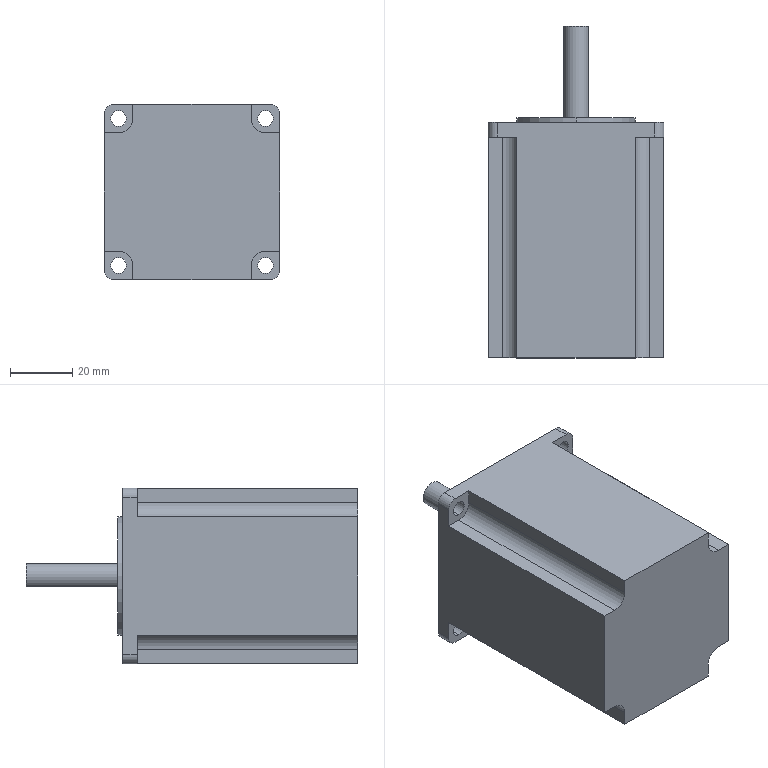Part | SolidWorks | features BaseBody 1 | 1 solid | 40 faces | box 56.4 x 106.5 x 56.4 mm | volume 220040 mm3 | plane 21 | cylinder 19 | commonest cylinder face diameters 5 x8 6 x4 9.26 x4 38.1 x2 8 x1
STEP:
#1=CARTESIAN_POINT('',(1.936,77.1,-3.5));
#2=VERTEX_POINT('',#1);
#3=CARTESIAN_POINT('',(-1.936,77.1,-3.5));
#4=VERTEX_POINT('',#3);
#5=CARTESIAN_POINT('',(1.936,77.1,-3.5));
#6=DIRECTION('',(-1.,0.,0.));
#7=VECTOR('',#6,1000.);
#8=LINE('',#5,#7);
#9=EDGE_CURVE('',#2,#4,#8,.T.);
#10=ORIENTED_EDGE('',*,*,#9,.T.);
#11=CARTESIAN_POINT('',(-1.936,106.5,-3.5));
#12=VERTEX_POINT('',#11);
#13=CARTESIAN_POINT('',(-1.936,73.195,-3.5));
#14=DIRECTION('',(0.,1.,0.));
#15=VECTOR('',#14,1000.);
#16=LINE('',#13,#15);
#17=EDGE_CURVE('',#4,#12,#16,.T.);
#18=ORIENTED_EDGE('',*,*,#17,.T.);
#19=CARTESIAN_POINT('',(1.936,106.5,-3.5));
#20=VERTEX_POINT('',#19);
#21=CARTESIAN_POINT('',(1.936,106.5,-3.5));
#22=DIRECTION('',(1.,0.,0.));
#23=VECTOR('',#22,1000.);
#24=LINE('',#21,#23);
#25=EDGE_CURVE('',#12,#20,#24,.T.);
#26=ORIENTED_EDGE('',*,*,#25,.T.);
#27=CARTESIAN_POINT('',(1.936,73.195,-3.5));
#28=DIRECTION('',(0.,1.,0.));
#29=VECTOR('',#28,1000.);
#30=LINE('',#27,#29);
#31=EDGE_CURVE('',#2,#20,#30,.T.);
#32=ORIENTED_EDGE('',*,*,#31,.F.);
#33=EDGE_LOOP('',(#10,#18,#26,#32));
#34=FACE_OUTER_BOUND('',#33,.T.);
#35=CARTESIAN_POINT('',(1.936,73.195,-3.5));
#36=DIRECTION('',(0.,0.,1.));
#37=DIRECTION('',(1.,0.,0.));
#38=AXIS2_PLACEMENT_3D('',#35,#36,#37);
#39=PLANE('',#38);
#40=ADVANCED_FACE('',(#34),#39,.F.);
#41=CARTESIAN_POINT('',(23.57,70.8,21.07));
#42=VERTEX_POINT('',#41);
#43=CARTESIAN_POINT('',(23.57,75.5,21.07));
#44=VERTEX_POINT('',#43);
#45=CARTESIAN_POINT('',(23.57,0.,21.07));
#46=DIRECTION('',(0.,1.,0.));
#47=VECTOR('',#46,1000.);
#48=LINE('',#45,#47);
#49=EDGE_CURVE('',#42,#44,#48,.T.);
#50=ORIENTED_EDGE('',*,*,#49,.F.);
#51=CARTESIAN_POINT('',(23.57,70.8,26.07));
#52=VERTEX_POINT('',#51);
#53=CARTESIAN_POINT('',(23.57,70.8,23.57));
#54=DIRECTION('',(0.,1.,0.));
#55=DIRECTION('',(0.,0.,1.));
#56=AXIS2_PLACEMENT_3D('',#53,#54,#55);
#57=CIRCLE('',#56,2.5);
#58=EDGE_CURVE('',#52,#42,#57,.T.);
#59=ORIENTED_EDGE('',*,*,#58,.F.);
#60=CARTESIAN_POINT('',(23.57,75.5,26.07));
#61=VERTEX_POINT('',#60);
#62=CARTESIAN_POINT('',(23.57,0.,26.07));
#63=DIRECTION('',(0.,1.,0.));
#64=VECTOR('',#63,1000.);
#65=LINE('',#62,#64);
#66=EDGE_CURVE('',#52,#61,#65,.T.);
#67=ORIENTED_EDGE('',*,*,#66,.T.);
#68=CARTESIAN_POINT('',(23.57,75.5,23.57));
#69=DIRECTION('',(0.,1.,0.));
#70=DIRECTION('',(0.,0.,1.));
#71=AXIS2_PLACEMENT_3D('',#68,#69,#70);
#72=CIRCLE('',#71,2.5);
#73=EDGE_CURVE('',#61,#44,#72,.T.);
#74=ORIENTED_EDGE('',*,*,#73,.T.);
#75=EDGE_LOOP('',(#50,#59,#67,#74));
#76=FACE_OUTER_BOUND('',#75,.T.);
#77=CARTESIAN_POINT('',(23.57,0.,23.57));
#78=DIRECTION('',(0.,1.,0.));
#79=DIRECTION('',(0.,0.,1.));
#80=AXIS2_PLACEMENT_3D('',#77,#78,#79);
#81=CYLINDRICAL_SURFACE('',#80,2.5);
#82=ADVANCED_FACE('',(#76),#81,.F.);
#83=CARTESIAN_POINT('',(-23.57,70.8,-26.07));
#84=VERTEX_POINT('',#83);
#85=CARTESIAN_POINT('',(-23.57,75.5,-26.07));
#86=VERTEX_POINT('',#85);
#87=CARTESIAN_POINT('',(-23.57,0.,-26.07));
#88=DIRECTION('',(0.,1.,0.));
#89=VECTOR('',#88,1000.);
#90=LINE('',#87,#89);
#91=EDGE_CURVE('',#84,#86,#90,.T.);
#92=ORIENTED_EDGE('',*,*,#91,.F.);
#93=CARTESIAN_POINT('',(-23.57,70.8,-21.07));
#94=VERTEX_POINT('',#93);
#95=CARTESIAN_POINT('',(-23.57,70.8,-23.57));
#96=DIRECTION('',(0.,1.,0.));
#97=DIRECTION('',(0.,0.,1.));
#98=AXIS2_PLACEMENT_3D('',#95,#96,#97);
#99=CIRCLE('',#98,2.5);
#100=EDGE_CURVE('',#94,#84,#99,.T.);
#101=ORIENTED_EDGE('',*,*,#100,.F.);
#102=CARTESIAN_POINT('',(-23.57,75.5,-21.07));
#103=VERTEX_POINT('',#102);
#104=CARTESIAN_POINT('',(-23.57,0.,-21.07));
#105=DIRECTION('',(0.,1.,0.));
#106=VECTOR('',#105,1000.);
#107=LINE('',#104,#106);
#108=EDGE_CURVE('',#94,#103,#107,.T.);
#109=ORIENTED_EDGE('',*,*,#108,.T.);
#110=CARTESIAN_POINT('',(-23.57,75.5,-23.57));
#111=DIRECTION('',(0.,1.,0.));
#112=DIRECTION('',(0.,0.,1.));
#113=AXIS2_PLACEMENT_3D('',#110,#111,#112);
#114=CIRCLE('',#113,2.5);
#115=EDGE_CURVE('',#103,#86,#114,.T.);
#116=ORIENTED_EDGE('',*,*,#115,.T.);
#117=EDGE_LOOP('',(#92,#101,#109,#116));
#118=FACE_OUTER_BOUND('',#117,.T.);
#119=CARTESIAN_POINT('',(-23.57,0.,-23.57));
#120=DIRECTION('',(0.,1.,0.));
#121=DIRECTION('',(0.,0.,1.));
#122=AXIS2_PLACEMENT_3D('',#119,#120,#121);
#123=CYLINDRICAL_SURFACE('',#122,2.5);
#124=ADVANCED_FACE('',(#118),#123,.F.);
#125=CARTESIAN_POINT('',(23.57,70.8,-26.07));
#126=VERTEX_POINT('',#125);
#127=CARTESIAN_POINT('',(23.57,75.5,-26.07));
#128=VERTEX_POINT('',#127);
#129=CARTESIAN_POINT('',(23.57,0.,-26.07));
#130=DIRECTION('',(0.,1.,0.));
#131=VECTOR('',#130,1000.);
#132=LINE('',#129,#131);
#133=EDGE_CURVE('',#126,#128,#132,.T.);
#134=ORIENTED_EDGE('',*,*,#133,.F.);
#135=CARTESIAN_POINT('',(23.57,70.8,-21.07));
#136=VERTEX_POINT('',#135);
#137=CARTESIAN_POINT('',(23.57,70.8,-23.57));
#138=DIRECTION('',(0.,-1.,0.));
#139=DIRECTION('',(0.,0.,-1.));
#140=AXIS2_PLACEMENT_3D('',#137,#138,#139);
#141=CIRCLE('',#140,2.5);
#142=EDGE_CURVE('',#126,#136,#141,.T.);
#143=ORIENTED_EDGE('',*,*,#142,.T.);
#144=CARTESIAN_POINT('',(23.57,75.5,-21.07));
#145=VERTEX_POINT('',#144);
#146=CARTESIAN_POINT('',(23.57,0.,-21.07));
#147=DIRECTION('',(0.,1.,0.));
#148=VECTOR('',#147,1000.);
#149=LINE('',#146,#148);
#150=EDGE_CURVE('',#136,#145,#149,.T.);
#151=ORIENTED_EDGE('',*,*,#150,.T.);
#152=CARTESIAN_POINT('',(23.57,75.5,-23.57));
#153=DIRECTION('',(0.,1.,0.));
#154=DIRECTION('',(0.,0.,-1.));
#155=AXIS2_PLACEMENT_3D('',#152,#153,#154);
#156=CIRCLE('',#155,2.5);
#157=EDGE_CURVE('',#145,#128,#156,.T.);
#158=ORIENTED_EDGE('',*,*,#157,.T.);
#159=EDGE_LOOP('',(#134,#143,#151,#158));
#160=FACE_OUTER_BOUND('',#159,.T.);
#161=CARTESIAN_POINT('',(23.57,0.,-23.57));
#162=DIRECTION('',(0.,1.,0.));
#163=DIRECTION('',(0.,0.,1.));
#164=AXIS2_PLACEMENT_3D('',#161,#162,#163);
#165=CYLINDRICAL_SURFACE('',#164,2.5);
#166=ADVANCED_FACE('',(#160),#165,.F.);
#167=CARTESIAN_POINT('',(-23.57,70.8,21.07));
#168=VERTEX_POINT('',#167);
#169=CARTESIAN_POINT('',(-23.57,75.5,21.07));
#170=VERTEX_POINT('',#169);
#171=CARTESIAN_POINT('',(-23.57,0.,21.07));
#172=DIRECTION('',(0.,1.,0.));
#173=VECTOR('',#172,1000.);
#174=LINE('',#171,#173);
#175=EDGE_CURVE('',#168,#170,#174,.T.);
#176=ORIENTED_EDGE('',*,*,#175,.F.);
#177=CARTESIAN_POINT('',(-23.57,70.8,26.07));
#178=VERTEX_POINT('',#177);
#179=CARTESIAN_POINT('',(-23.57,70.8,23.57));
#180=DIRECTION('',(0.,-1.,0.));
#181=DIRECTION('',(0.,0.,-1.));
#182=AXIS2_PLACEMENT_3D('',#179,#180,#181);
#183=CIRCLE('',#182,2.5);
#184=EDGE_CURVE('',#168,#178,#183,.T.);
#185=ORIENTED_EDGE('',*,*,#184,.T.);
#186=CARTESIAN_POINT('',(-23.57,75.5,26.07));
#187=VERTEX_POINT('',#186);
#188=CARTESIAN_POINT('',(-23.57,0.,26.07));
#189=DIRECTION('',(0.,1.,0.));
#190=VECTOR('',#189,1000.);
#191=LINE('',#188,#190);
#192=EDGE_CURVE('',#178,#187,#191,.T.);
#193=ORIENTED_EDGE('',*,*,#192,.T.);
#194=CARTESIAN_POINT('',(-23.57,75.5,23.57));
#195=DIRECTION('',(0.,1.,0.));
#196=DIRECTION('',(0.,0.,-1.));
#197=AXIS2_PLACEMENT_3D('',#194,#195,#196);
#198=CIRCLE('',#197,2.5);
#199=EDGE_CURVE('',#187,#170,#198,.T.);
#200=ORIENTED_EDGE('',*,*,#199,.T.);
#201=EDGE_LOOP('',(#176,#185,#193,#200));
#202=FACE_OUTER_BOUND('',#201,.T.);
#203=CARTESIAN_POINT('',(-23.57,0.,23.57));
#204=DIRECTION('',(0.,1.,0.));
#205=DIRECTION('',(0.,0.,1.));
#206=AXIS2_PLACEMENT_3D('',#203,#204,#205);
#207=CYLINDRICAL_SURFACE('',#206,2.5);
#208=ADVANCED_FACE('',(#202),#207,.F.);
#209=CARTESIAN_POINT('',(-28.2,75.5,25.2));
#210=VERTEX_POINT('',#209);
#211=CARTESIAN_POINT('',(-25.2,75.5,28.2));
#212=VERTEX_POINT('',#211);
#213=CARTESIAN_POINT('',(-25.2,75.5,25.2));
#214=DIRECTION('',(0.,1.,0.));
#215=DIRECTION('',(0.,0.,1.));
#216=AXIS2_PLACEMENT_3D('',#213,#214,#215);
#217=CIRCLE('',#216,3.);
#218=EDGE_CURVE('',#210,#212,#217,.T.);
#219=ORIENTED_EDGE('',*,*,#218,.F.);
#220=CARTESIAN_POINT('',(-28.2,70.8,25.2));
#221=VERTEX_POINT('',#220);
#222=CARTESIAN_POINT('',(-28.2,75.5,25.2));
#223=DIRECTION('',(0.,1.,0.));
#224=VECTOR('',#223,1000.);
#225=LINE('',#222,#224);
#226=EDGE_CURVE('',#221,#210,#225,.T.);
#227=ORIENTED_EDGE('',*,*,#226,.F.);
#228=CARTESIAN_POINT('',(-25.2,70.8,28.2));
#229=VERTEX_POINT('',#228);
#230=CARTESIAN_POINT('',(-25.2,70.8,25.2));
#231=DIRECTION('',(0.,-1.,0.));
#232=DIRECTION('',(0.,0.,-1.));
#233=AXIS2_PLACEMENT_3D('',#230,#231,#232);
#234=CIRCLE('',#233,3.);
#235=EDGE_CURVE('',#229,#221,#234,.T.);
#236=ORIENTED_EDGE('',*,*,#235,.F.);
#237=CARTESIAN_POINT('',(-25.2,75.5,28.2));
#238=DIRECTION('',(0.,-1.,0.));
#239=VECTOR('',#238,1000.);
#240=LINE('',#237,#239);
#241=EDGE_CURVE('',#212,#229,#240,.T.);
#242=ORIENTED_EDGE('',*,*,#241,.F.);
#243=EDGE_LOOP('',(#219,#227,#236,#242));
#244=FACE_OUTER_BOUND('',#243,.T.);
#245=CARTESIAN_POINT('',(-25.2,75.5,25.2));
#246=DIRECTION('',(0.,-1.,0.));
#247=DIRECTION('',(0.,0.,-1.));
#248=AXIS2_PLACEMENT_3D('',#245,#246,#247);
#249=CYLINDRICAL_SURFACE('',#248,3.);
#250=ADVANCED_FACE('',(#244),#249,.T.);
#251=CARTESIAN_POINT('',(-25.2,75.5,-28.2));
#252=VERTEX_POINT('',#251);
#253=CARTESIAN_POINT('',(-28.2,75.5,-25.2));
#254=VERTEX_POINT('',#253);
#255=CARTESIAN_POINT('',(-25.2,75.5,-25.2));
#256=DIRECTION('',(0.,1.,0.));
#257=DIRECTION('',(0.,0.,1.));
#258=AXIS2_PLACEMENT_3D('',#255,#256,#257);
#259=CIRCLE('',#258,3.);
#260=EDGE_CURVE('',#252,#254,#259,.T.);
#261=ORIENTED_EDGE('',*,*,#260,.F.);
#262=CARTESIAN_POINT('',(-25.2,70.8,-28.2));
#263=VERTEX_POINT('',#262);
#264=CARTESIAN_POINT('',(-25.2,75.5,-28.2));
#265=DIRECTION('',(0.,1.,0.));
#266=VECTOR('',#265,1000.);
#267=LINE('',#264,#266);
#268=EDGE_CURVE('',#263,#252,#267,.T.);
#269=ORIENTED_EDGE('',*,*,#268,.F.);
#270=CARTESIAN_POINT('',(-28.2,70.8,-25.2));
#271=VERTEX_POINT('',#270);
#272=CARTESIAN_POINT('',(-25.2,70.8,-25.2));
#273=DIRECTION('',(0.,-1.,0.));
#274=DIRECTION('',(0.,0.,1.));
#275=AXIS2_PLACEMENT_3D('',#272,#273,#274);
#276=CIRCLE('',#275,3.);
#277=EDGE_CURVE('',#271,#263,#276,.T.);
#278=ORIENTED_EDGE('',*,*,#277,.F.);
#279=CARTESIAN_POINT('',(-28.2,75.5,-25.2));
#280=DIRECTION('',(0.,-1.,0.));
#281=VECTOR('',#280,1000.);
#282=LINE('',#279,#281);
#283=EDGE_CURVE('',#254,#271,#282,.T.);
#284=ORIENTED_EDGE('',*,*,#283,.F.);
#285=EDGE_LOOP('',(#261,#269,#278,#284));
#286=FACE_OUTER_BOUND('',#285,.T.);
#287=CARTESIAN_POINT('',(-25.2,75.5,-25.2));
#288=DIRECTION('',(0.,-1.,0.));
#289=DIRECTION('',(0.,0.,-1.));
#290=AXIS2_PLACEMENT_3D('',#287,#288,#289);
#291=CYLINDRICAL_SURFACE('',#290,3.);
#292=ADVANCED_FACE('',(#286),#291,.T.);
#293=CARTESIAN_POINT('',(25.2,75.5,28.2));
#294=VERTEX_POINT('',#293);
#295=CARTESIAN_POINT('',(28.2,75.5,25.2));
#296=VERTEX_POINT('',#295);
#297=CARTESIAN_POINT('',(25.2,75.5,25.2));
#298=DIRECTION('',(0.,1.,0.));
#299=DIRECTION('',(0.,0.,1.));
#300=AXIS2_PLACEMENT_3D('',#297,#298,#299);
#301=CIRCLE('',#300,3.);
#302=EDGE_CURVE('',#294,#296,#301,.T.);
#303=ORIENTED_EDGE('',*,*,#302,.F.);
#304=CARTESIAN_POINT('',(25.2,70.8,28.2));
#305=VERTEX_POINT('',#304);
#306=CARTESIAN_POINT('',(25.2,75.5,28.2));
#307=DIRECTION('',(0.,1.,0.));
#308=VECTOR('',#307,1000.);
#309=LINE('',#306,#308);
#310=EDGE_CURVE('',#305,#294,#309,.T.);
#311=ORIENTED_EDGE('',*,*,#310,.F.);
#312=CARTESIAN_POINT('',(28.2,70.8,25.2));
#313=VERTEX_POINT('',#312);
#314=CARTESIAN_POINT('',(25.2,70.8,25.2));
#315=DIRECTION('',(0.,-1.,0.));
#316=DIRECTION('',(0.,0.,1.));
#317=AXIS2_PLACEMENT_3D('',#314,#315,#316);
#318=CIRCLE('',#317,3.);
#319=EDGE_CURVE('',#313,#305,#318,.T.);
#320=ORIENTED_EDGE('',*,*,#319,.F.);
#321=CARTESIAN_POINT('',(28.2,75.5,25.2));
#322=DIRECTION('',(0.,-1.,0.));
#323=VECTOR('',#322,1000.);
#324=LINE('',#321,#323);
#325=EDGE_CURVE('',#296,#313,#324,.T.);
#326=ORIENTED_EDGE('',*,*,#325,.F.);
#327=EDGE_LOOP('',(#303,#311,#320,#326));
#328=FACE_OUTER_BOUND('',#327,.T.);
#329=CARTESIAN_POINT('',(25.2,75.5,25.2));
#330=DIRECTION('',(0.,-1.,0.));
#331=DIRECTION('',(0.,0.,-1.));
#332=AXIS2_PLACEMENT_3D('',#329,#330,#331);
#333=CYLINDRICAL_SURFACE('',#332,3.);
#334=ADVANCED_FACE('',(#328),#333,.T.);
#335=CARTESIAN_POINT('',(28.2,75.5,-25.2));
#336=VERTEX_POINT('',#335);
#337=CARTESIAN_POINT('',(25.2,75.5,-28.2));
#338=VERTEX_POINT('',#337);
#339=CARTESIAN_POINT('',(25.2,75.5,-25.2));
#340=DIRECTION('',(0.,1.,0.));
#341=DIRECTION('',(0.,0.,1.));
#342=AXIS2_PLACEMENT_3D('',#339,#340,#341);
#343=CIRCLE('',#342,3.);
#344=EDGE_CURVE('',#336,#338,#343,.T.);
#345=ORIENTED_EDGE('',*,*,#344,.F.);
#346=CARTESIAN_POINT('',(28.2,70.8,-25.2));
#347=VERTEX_POINT('',#346);
#348=CARTESIAN_POINT('',(28.2,75.5,-25.2));
#349=DIRECTION('',(0.,1.,0.));
#350=VECTOR('',#349,1000.);
#351=LINE('',#348,#350);
#352=EDGE_CURVE('',#347,#336,#351,.T.);
#353=ORIENTED_EDGE('',*,*,#352,.F.);
#354=CARTESIAN_POINT('',(25.2,70.8,-28.2));
#355=VERTEX_POINT('',#354);
#356=CARTESIAN_POINT('',(25.2,70.8,-25.2));
#357=DIRECTION('',(0.,-1.,0.));
#358=DIRECTION('',(0.,0.,-1.));
#359=AXIS2_PLACEMENT_3D('',#356,#357,#358);
#360=CIRCLE('',#359,3.);
#361=EDGE_CURVE('',#355,#347,#360,.T.);
#362=ORIENTED_EDGE('',*,*,#361,.F.);
#363=CARTESIAN_POINT('',(25.2,75.5,-28.2));
#364=DIRECTION('',(0.,-1.,0.));
#365=VECTOR('',#364,1000.);
#366=LINE('',#363,#365);
#367=EDGE_CURVE('',#338,#355,#366,.T.);
#368=ORIENTED_EDGE('',*,*,#367,.F.);
#369=EDGE_LOOP('',(#345,#353,#362,#368));
#370=FACE_OUTER_BOUND('',#369,.T.);
#371=CARTESIAN_POINT('',(25.2,75.5,-25.2));
#372=DIRECTION('',(0.,-1.,0.));
#373=DIRECTION('',(0.,0.,-1.));
#374=AXIS2_PLACEMENT_3D('',#371,#372,#373);
#375=CYLINDRICAL_SURFACE('',#374,3.);
#376=ADVANCED_FACE('',(#370),#375,.T.);
#377=CARTESIAN_POINT('',(-23.57,70.8,23.57));
#378=DIRECTION('',(0.,-1.,0.));
#379=DIRECTION('',(0.,0.,-1.));
#380=AXIS2_PLACEMENT_3D('',#377,#378,#379);
#381=CIRCLE('',#380,2.5);
#382=EDGE_CURVE('',#178,#168,#381,.T.);
#383=ORIENTED_EDGE('',*,*,#382,.F.);
#384=ORIENTED_EDGE('',*,*,#184,.F.);
#385=EDGE_LOOP('',(#383,#384));
#386=FACE_BOUND('',#385,.T.);
#387=CARTESIAN_POINT('',(-18.94,70.8,28.2));
#388=VERTEX_POINT('',#387);
#389=CARTESIAN_POINT('',(-28.2,70.8,28.2));
#390=DIRECTION('',(-1.,0.,0.));
#391=VECTOR('',#390,1000.);
#392=LINE('',#389,#391);
#393=EDGE_CURVE('',#388,#229,#392,.T.);
#394=ORIENTED_EDGE('',*,*,#393,.T.);
#395=ORIENTED_EDGE('',*,*,#235,.T.);
#396=CARTESIAN_POINT('',(-28.2,70.8,18.94));
#397=VERTEX_POINT('',#396);
#398=CARTESIAN_POINT('',(-28.2,70.8,18.94));
#399=DIRECTION('',(0.,0.,-1.));
#400=VECTOR('',#399,1000.);
#401=LINE('',#398,#400);
#402=EDGE_CURVE('',#221,#397,#401,.T.);
#403=ORIENTED_EDGE('',*,*,#402,.T.);
#404=CARTESIAN_POINT('',(-23.57,70.8,18.94));
#405=VERTEX_POINT('',#404);
#406=CARTESIAN_POINT('',(-23.57,70.8,18.94));
#407=DIRECTION('',(1.,0.,0.));
#408=VECTOR('',#407,1000.);
#409=LINE('',#406,#408);
#410=EDGE_CURVE('',#397,#405,#409,.T.);
#411=ORIENTED_EDGE('',*,*,#410,.T.);
#412=CARTESIAN_POINT('',(-18.94,70.8,23.57));
#413=VERTEX_POINT('',#412);
#414=CARTESIAN_POINT('',(-23.57,70.8,23.57));
#415=DIRECTION('',(0.,-1.,0.));
#416=DIRECTION('',(0.,0.,-1.));
#417=AXIS2_PLACEMENT_3D('',#414,#415,#416);
#418=CIRCLE('',#417,4.63);
#419=EDGE_CURVE('',#405,#413,#418,.T.);
#420=ORIENTED_EDGE('',*,*,#419,.T.);
#421=CARTESIAN_POINT('',(-18.94,70.8,23.57));
#422=DIRECTION('',(0.,0.,1.));
#423=VECTOR('',#422,1000.);
#424=LINE('',#421,#423);
#425=EDGE_CURVE('',#413,#388,#424,.T.);
#426=ORIENTED_EDGE('',*,*,#425,.T.);
#427=EDGE_LOOP('',(#394,#395,#403,#411,#420,#426));
#428=FACE_OUTER_BOUND('',#427,.T.);
#429=CARTESIAN_POINT('',(-23.57,70.8,23.57));
#430=DIRECTION('',(0.,-1.,0.));
#431=DIRECTION('',(0.,0.,-1.));
#432=AXIS2_PLACEMENT_3D('',#429,#430,#431);
#433=PLANE('',#432);
#434=ADVANCED_FACE('',(#386,#428),#433,.T.);
#435=CARTESIAN_POINT('',(-18.94,0.,23.57));
#436=VERTEX_POINT('',#435);
#437=CARTESIAN_POINT('',(-18.94,0.,28.2));
#438=VERTEX_POINT('',#437);
#439=CARTESIAN_POINT('',(-18.94,0.,23.57));
#440=DIRECTION('',(0.,0.,1.));
#441=VECTOR('',#440,1000.);
#442=LINE('',#439,#441);
#443=EDGE_CURVE('',#436,#438,#442,.T.);
#444=ORIENTED_EDGE('',*,*,#443,.T.);
#445=CARTESIAN_POINT('',(-18.94,70.8,28.2));
#446=DIRECTION('',(0.,-1.,0.));
#447=VECTOR('',#446,1000.);
#448=LINE('',#445,#447);
#449=EDGE_CURVE('',#388,#438,#448,.T.);
#450=ORIENTED_EDGE('',*,*,#449,.F.);
#451=ORIENTED_EDGE('',*,*,#425,.F.);
#452=CARTESIAN_POINT('',(-18.94,70.8,23.57));
#453=DIRECTION('',(0.,-1.,0.));
#454=VECTOR('',#453,1000.);
#455=LINE('',#452,#454);
#456=EDGE_CURVE('',#413,#436,#455,.T.);
#457=ORIENTED_EDGE('',*,*,#456,.T.);
#458=EDGE_LOOP('',(#444,#450,#451,#457));
#459=FACE_OUTER_BOUND('',#458,.T.);
#460=CARTESIAN_POINT('',(-18.94,70.8,23.57));
#461=DIRECTION('',(1.,0.,0.));
#462=DIRECTION('',(0.,0.,1.));
#463=AXIS2_PLACEMENT_3D('',#460,#461,#462);
#464=PLANE('',#463);
#465=ADVANCED_FACE('',(#459),#464,.F.);
#466=CARTESIAN_POINT('',(-28.2,0.,18.94));
#467=VERTEX_POINT('',#466);
#468=CARTESIAN_POINT('',(-23.57,0.,18.94));
#469=VERTEX_POINT('',#468);
#470=CARTESIAN_POINT('',(-23.57,0.,18.94));
#471=DIRECTION('',(1.,0.,0.));
#472=VECTOR('',#471,1000.);
#473=LINE('',#470,#472);
#474=EDGE_CURVE('',#467,#469,#473,.T.);
#475=ORIENTED_EDGE('',*,*,#474,.T.);
#476=CARTESIAN_POINT('',(-23.57,70.8,18.94));
#477=DIRECTION('',(0.,-1.,0.));
#478=VECTOR('',#477,1000.);
#479=LINE('',#476,#478);
#480=EDGE_CURVE('',#405,#469,#479,.T.);
#481=ORIENTED_EDGE('',*,*,#480,.F.);
#482=ORIENTED_EDGE('',*,*,#410,.F.);
#483=CARTESIAN_POINT('',(-28.2,70.8,18.94));
#484=DIRECTION('',(0.,-1.,0.));
#485=VECTOR('',#484,1000.);
#486=LINE('',#483,#485);
#487=EDGE_CURVE('',#397,#467,#486,.T.);
#488=ORIENTED_EDGE('',*,*,#487,.T.);
#489=EDGE_LOOP('',(#475,#481,#482,#488));
#490=FACE_OUTER_BOUND('',#489,.T.);
#491=CARTESIAN_POINT('',(-23.57,70.8,18.94));
#492=DIRECTION('',(0.,0.,-1.));
#493=DIRECTION('',(0.,-1.,0.));
#494=AXIS2_PLACEMENT_3D('',#491,#492,#493);
#495=PLANE('',#494);
#496=ADVANCED_FACE('',(#490),#495,.F.);
#497=CARTESIAN_POINT('',(-23.57,0.,23.57));
#498=DIRECTION('',(0.,-1.,0.));
#499=DIRECTION('',(0.,0.,-1.));
#500=AXIS2_PLACEMENT_3D('',#497,#498,#499);
#501=CIRCLE('',#500,4.63);
#502=EDGE_CURVE('',#469,#436,#501,.T.);
#503=ORIENTED_EDGE('',*,*,#502,.T.);
#504=ORIENTED_EDGE('',*,*,#456,.F.);
#505=ORIENTED_EDGE('',*,*,#419,.F.);
#506=ORIENTED_EDGE('',*,*,#480,.T.);
#507=EDGE_LOOP('',(#503,#504,#505,#506));
#508=FACE_OUTER_BOUND('',#507,.T.);
#509=CARTESIAN_POINT('',(-23.57,70.8,23.57));
#510=DIRECTION('',(0.,-1.,0.));
#511=DIRECTION('',(0.,0.,-1.));
#512=AXIS2_PLACEMENT_3D('',#509,#510,#511);
#513=CYLINDRICAL_SURFACE('',#512,4.63);
#514=ADVANCED_FACE('',(#508),#513,.F.);
#515=CARTESIAN_POINT('',(23.57,70.8,-23.57));
#516=DIRECTION('',(0.,-1.,0.));
#517=DIRECTION('',(0.,0.,-1.));
#518=AXIS2_PLACEMENT_3D('',#515,#516,#517);
#519=CIRCLE('',#518,2.5);
#520=EDGE_CURVE('',#136,#126,#519,.T.);
#521=ORIENTED_EDGE('',*,*,#520,.F.);
#522=ORIENTED_EDGE('',*,*,#142,.F.);
#523=EDGE_LOOP('',(#521,#522));
#524=FACE_BOUND('',#523,.T.);
#525=CARTESIAN_POINT('',(18.94,70.8,-28.2));
#526=VERTEX_POINT('',#525);
#527=CARTESIAN_POINT('',(28.2,70.8,-28.2));
#528=DIRECTION('',(1.,0.,0.));
#529=VECTOR('',#528,1000.);
#530=LINE('',#527,#529);
#531=EDGE_CURVE('',#526,#355,#530,.T.);
#532=ORIENTED_EDGE('',*,*,#531,.T.);
#533=ORIENTED_EDGE('',*,*,#361,.T.);
#534=CARTESIAN_POINT('',(28.2,70.8,-18.94));
#535=VERTEX_POINT('',#534);
#536=CARTESIAN_POINT('',(28.2,70.8,-18.94));
#537=DIRECTION('',(0.,0.,1.));
#538=VECTOR('',#537,1000.);
#539=LINE('',#536,#538);
#540=EDGE_CURVE('',#347,#535,#539,.T.);
#541=ORIENTED_EDGE('',*,*,#540,.T.);
#542=CARTESIAN_POINT('',(23.57,70.8,-18.94));
#543=VERTEX_POINT('',#542);
#544=CARTESIAN_POINT('',(23.57,70.8,-18.94));
#545=DIRECTION('',(-1.,0.,0.));
#546=VECTOR('',#545,1000.);
#547=LINE('',#544,#546);
#548=EDGE_CURVE('',#535,#543,#547,.T.);
#549=ORIENTED_EDGE('',*,*,#548,.T.);
#550=CARTESIAN_POINT('',(18.94,70.8,-23.57));
#551=VERTEX_POINT('',#550);
#552=CARTESIAN_POINT('',(23.57,70.8,-23.57));
#553=DIRECTION('',(0.,-1.,0.));
#554=DIRECTION('',(0.,0.,-1.));
#555=AXIS2_PLACEMENT_3D('',#552,#553,#554);
#556=CIRCLE('',#555,4.63);
#557=EDGE_CURVE('',#543,#551,#556,.T.);
#558=ORIENTED_EDGE('',*,*,#557,.T.);
#559=CARTESIAN_POINT('',(18.94,70.8,-23.57));
#560=DIRECTION('',(0.,0.,-1.));
#561=VECTOR('',#560,1000.);
#562=LINE('',#559,#561);
#563=EDGE_CURVE('',#551,#526,#562,.T.);
#564=ORIENTED_EDGE('',*,*,#563,.T.);
#565=EDGE_LOOP('',(#532,#533,#541,#549,#558,#564));
#566=FACE_OUTER_BOUND('',#565,.T.);
#567=CARTESIAN_POINT('',(23.57,70.8,-23.57));
#568=DIRECTION('',(0.,-1.,0.));
#569=DIRECTION('',(0.,0.,-1.));
#570=AXIS2_PLACEMENT_3D('',#567,#568,#569);
#571=PLANE('',#570);
#572=ADVANCED_FACE('',(#524,#566),#571,.T.);
#573=CARTESIAN_POINT('',(18.94,0.,-23.57));
#574=VERTEX_POINT('',#573);
#575=CARTESIAN_POINT('',(18.94,0.,-28.2));
#576=VERTEX_POINT('',#575);
#577=CARTESIAN_POINT('',(18.94,0.,-23.57));
#578=DIRECTION('',(0.,0.,-1.));
#579=VECTOR('',#578,1000.);
#580=LINE('',#577,#579);
#581=EDGE_CURVE('',#574,#576,#580,.T.);
#582=ORIENTED_EDGE('',*,*,#581,.T.);
#583=CARTESIAN_POINT('',(18.94,70.8,-28.2));
#584=DIRECTION('',(0.,-1.,0.));
#585=VECTOR('',#584,1000.);
#586=LINE('',#583,#585);
#587=EDGE_CURVE('',#526,#576,#586,.T.);
#588=ORIENTED_EDGE('',*,*,#587,.F.);
#589=ORIENTED_EDGE('',*,*,#563,.F.);
#590=CARTESIAN_POINT('',(18.94,70.8,-23.57));
#591=DIRECTION('',(0.,-1.,0.));
#592=VECTOR('',#591,1000.);
#593=LINE('',#590,#592);
#594=EDGE_CURVE('',#551,#574,#593,.T.);
#595=ORIENTED_EDGE('',*,*,#594,.T.);
#596=EDGE_LOOP('',(#582,#588,#589,#595));
#597=FACE_OUTER_BOUND('',#596,.T.);
#598=CARTESIAN_POINT('',(18.94,70.8,-23.57));
#599=DIRECTION('',(-1.,0.,0.));
#600=DIRECTION('',(0.,0.,1.));
#601=AXIS2_PLACEMENT_3D('',#598,#599,#600);
#602=PLANE('',#601);
#603=ADVANCED_FACE('',(#597),#602,.F.);
#604=CARTESIAN_POINT('',(28.2,0.,-18.94));
#605=VERTEX_POINT('',#604);
#606=CARTESIAN_POINT('',(23.57,0.,-18.94));
#607=VERTEX_POINT('',#606);
#608=CARTESIAN_POINT('',(23.57,0.,-18.94));
#609=DIRECTION('',(-1.,0.,0.));
#610=VECTOR('',#609,1000.);
#611=LINE('',#608,#610);
#612=EDGE_CURVE('',#605,#607,#611,.T.);
#613=ORIENTED_EDGE('',*,*,#612,.T.);
#614=CARTESIAN_POINT('',(23.57,70.8,-18.94));
#615=DIRECTION('',(0.,-1.,0.));
#616=VECTOR('',#615,1000.);
#617=LINE('',#614,#616);
#618=EDGE_CURVE('',#543,#607,#617,.T.);
#619=ORIENTED_EDGE('',*,*,#618,.F.);
#620=ORIENTED_EDGE('',*,*,#548,.F.);
#621=CARTESIAN_POINT('',(28.2,70.8,-18.94));
#622=DIRECTION('',(0.,-1.,0.));
#623=VECTOR('',#622,1000.);
#624=LINE('',#621,#623);
#625=EDGE_CURVE('',#535,#605,#624,.T.);
#626=ORIENTED_EDGE('',*,*,#625,.T.);
#627=EDGE_LOOP('',(#613,#619,#620,#626));
#628=FACE_OUTER_BOUND('',#627,.T.);
#629=CARTESIAN_POINT('',(23.57,70.8,-18.94));
#630=DIRECTION('',(0.,0.,1.));
#631=DIRECTION('',(1.,0.,0.));
#632=AXIS2_PLACEMENT_3D('',#629,#630,#631);
#633=PLANE('',#632);
#634=ADVANCED_FACE('',(#628),#633,.F.);
#635=CARTESIAN_POINT('',(23.57,0.,-23.57));
#636=DIRECTION('',(0.,-1.,0.));
#637=DIRECTION('',(0.,0.,-1.));
#638=AXIS2_PLACEMENT_3D('',#635,#636,#637);
#639=CIRCLE('',#638,4.63);
#640=EDGE_CURVE('',#607,#574,#639,.T.);
#641=ORIENTED_EDGE('',*,*,#640,.T.);
#642=ORIENTED_EDGE('',*,*,#594,.F.);
#643=ORIENTED_EDGE('',*,*,#557,.F.);
#644=ORIENTED_EDGE('',*,*,#618,.T.);
#645=EDGE_LOOP('',(#641,#642,#643,#644));
#646=FACE_OUTER_BOUND('',#645,.T.);
#647=CARTESIAN_POINT('',(23.57,70.8,-23.57));
#648=DIRECTION('',(0.,-1.,0.));
#649=DIRECTION('',(0.,0.,-1.));
#650=AXIS2_PLACEMENT_3D('',#647,#648,#649);
#651=CYLINDRICAL_SURFACE('',#650,4.63);
#652=ADVANCED_FACE('',(#646),#651,.F.);
#653=ORIENTED_EDGE('',*,*,#100,.T.);
#654=CARTESIAN_POINT('',(-23.57,70.8,-23.57));
#655=DIRECTION('',(0.,1.,0.));
#656=DIRECTION('',(0.,0.,1.));
#657=AXIS2_PLACEMENT_3D('',#654,#655,#656);
#658=CIRCLE('',#657,2.5);
#659=EDGE_CURVE('',#84,#94,#658,.T.);
#660=ORIENTED_EDGE('',*,*,#659,.T.);
#661=EDGE_LOOP('',(#653,#660));
#662=FACE_BOUND('',#661,.T.);
#663=CARTESIAN_POINT('',(-28.2,70.8,-18.94));
#664=VERTEX_POINT('',#663);
#665=CARTESIAN_POINT('',(-28.2,70.8,-18.94));
#666=DIRECTION('',(0.,0.,-1.));
#667=VECTOR('',#666,1000.);
#668=LINE('',#665,#667);
#669=EDGE_CURVE('',#664,#271,#668,.T.);
#670=ORIENTED_EDGE('',*,*,#669,.T.);
#671=ORIENTED_EDGE('',*,*,#277,.T.);
#672=CARTESIAN_POINT('',(-18.94,70.8,-28.2));
#673=VERTEX_POINT('',#672);
#674=CARTESIAN_POINT('',(-28.2,70.8,-28.2));
#675=DIRECTION('',(1.,0.,0.));
#676=VECTOR('',#675,1000.);
#677=LINE('',#674,#676);
#678=EDGE_CURVE('',#263,#673,#677,.T.);
#679=ORIENTED_EDGE('',*,*,#678,.T.);
#680=CARTESIAN_POINT('',(-18.94,70.8,-23.57));
#681=VERTEX_POINT('',#680);
#682=CARTESIAN_POINT('',(-18.94,70.8,-23.57));
#683=DIRECTION('',(0.,0.,1.));
#684=VECTOR('',#683,1000.);
#685=LINE('',#682,#684);
#686=EDGE_CURVE('',#673,#681,#685,.T.);
#687=ORIENTED_EDGE('',*,*,#686,.T.);
#688=CARTESIAN_POINT('',(-23.57,70.8,-18.94));
#689=VERTEX_POINT('',#688);
#690=CARTESIAN_POINT('',(-23.57,70.8,-23.57));
#691=DIRECTION('',(0.,-1.,0.));
#692=DIRECTION('',(0.,0.,1.));
#693=AXIS2_PLACEMENT_3D('',#690,#691,#692);
#694=CIRCLE('',#693,4.63);
#695=EDGE_CURVE('',#681,#689,#694,.T.);
#696=ORIENTED_EDGE('',*,*,#695,.T.);
#697=CARTESIAN_POINT('',(-23.57,70.8,-18.94));
#698=DIRECTION('',(-1.,0.,0.));
#699=VECTOR('',#698,1000.);
#700=LINE('',#697,#699);
#701=EDGE_CURVE('',#689,#664,#700,.T.);
#702=ORIENTED_EDGE('',*,*,#701,.T.);
#703=EDGE_LOOP('',(#670,#671,#679,#687,#696,#702));
#704=FACE_OUTER_BOUND('',#703,.T.);
#705=CARTESIAN_POINT('',(-23.57,70.8,-23.57));
#706=DIRECTION('',(0.,1.,0.));
#707=DIRECTION('',(1.,0.,0.));
#708=AXIS2_PLACEMENT_3D('',#705,#706,#707);
#709=PLANE('',#708);
#710=ADVANCED_FACE('',(#662,#704),#709,.F.);
#711=CARTESIAN_POINT('',(-23.57,0.,-18.94));
#712=VERTEX_POINT('',#711);
#713=CARTESIAN_POINT('',(-28.2,0.,-18.94));
#714=VERTEX_POINT('',#713);
#715=CARTESIAN_POINT('',(-23.57,0.,-18.94));
#716=DIRECTION('',(-1.,0.,0.));
#717=VECTOR('',#716,1000.);
#718=LINE('',#715,#717);
#719=EDGE_CURVE('',#712,#714,#718,.T.);
#720=ORIENTED_EDGE('',*,*,#719,.T.);
#721=CARTESIAN_POINT('',(-28.2,70.8,-18.94));
#722=DIRECTION('',(0.,-1.,0.));
#723=VECTOR('',#722,1000.);
#724=LINE('',#721,#723);
#725=EDGE_CURVE('',#664,#714,#724,.T.);
#726=ORIENTED_EDGE('',*,*,#725,.F.);
#727=ORIENTED_EDGE('',*,*,#701,.F.);
#728=CARTESIAN_POINT('',(-23.57,70.8,-18.94));
#729=DIRECTION('',(0.,-1.,0.));
#730=VECTOR('',#729,1000.);
#731=LINE('',#728,#730);
#732=EDGE_CURVE('',#689,#712,#731,.T.);
#733=ORIENTED_EDGE('',*,*,#732,.T.);
#734=EDGE_LOOP('',(#720,#726,#727,#733));
#735=FACE_OUTER_BOUND('',#734,.T.);
#736=CARTESIAN_POINT('',(-23.57,70.8,-18.94));
#737=DIRECTION('',(0.,0.,1.));
#738=DIRECTION('',(1.,0.,0.));
#739=AXIS2_PLACEMENT_3D('',#736,#737,#738);
#740=PLANE('',#739);
#741=ADVANCED_FACE('',(#735),#740,.F.);
#742=CARTESIAN_POINT('',(-18.94,0.,-28.2));
#743=VERTEX_POINT('',#742);
#744=CARTESIAN_POINT('',(-18.94,0.,-23.57));
#745=VERTEX_POINT('',#744);
#746=CARTESIAN_POINT('',(-18.94,0.,-23.57));
#747=DIRECTION('',(0.,0.,1.));
#748=VECTOR('',#747,1000.);
#749=LINE('',#746,#748);
#750=EDGE_CURVE('',#743,#745,#749,.T.);
#751=ORIENTED_EDGE('',*,*,#750,.T.);
#752=CARTESIAN_POINT('',(-18.94,70.8,-23.57));
#753=DIRECTION('',(0.,-1.,0.));
#754=VECTOR('',#753,1000.);
#755=LINE('',#752,#754);
#756=EDGE_CURVE('',#681,#745,#755,.T.);
#757=ORIENTED_EDGE('',*,*,#756,.F.);
#758=ORIENTED_EDGE('',*,*,#686,.F.);
#759=CARTESIAN_POINT('',(-18.94,70.8,-28.2));
#760=DIRECTION('',(0.,-1.,0.));
#761=VECTOR('',#760,1000.);
#762=LINE('',#759,#761);
#763=EDGE_CURVE('',#673,#743,#762,.T.);
#764=ORIENTED_EDGE('',*,*,#763,.T.);
#765=EDGE_LOOP('',(#751,#757,#758,#764));
#766=FACE_OUTER_BOUND('',#765,.T.);
#767=CARTESIAN_POINT('',(-18.94,70.8,-23.57));
#768=DIRECTION('',(1.,0.,0.));
#769=DIRECTION('',(0.,0.,-1.));
#770=AXIS2_PLACEMENT_3D('',#767,#768,#769);
#771=PLANE('',#770);
#772=ADVANCED_FACE('',(#766),#771,.F.);
#773=CARTESIAN_POINT('',(-23.57,0.,-23.57));
#774=DIRECTION('',(0.,-1.,0.));
#775=DIRECTION('',(0.,0.,1.));
#776=AXIS2_PLACEMENT_3D('',#773,#774,#775);
#777=CIRCLE('',#776,4.63);
#778=EDGE_CURVE('',#745,#712,#777,.T.);
#779=ORIENTED_EDGE('',*,*,#778,.T.);
#780=ORIENTED_EDGE('',*,*,#732,.F.);
#781=ORIENTED_EDGE('',*,*,#695,.F.);
#782=ORIENTED_EDGE('',*,*,#756,.T.);
#783=EDGE_LOOP('',(#779,#780,#781,#782));
#784=FACE_OUTER_BOUND('',#783,.T.);
#785=CARTESIAN_POINT('',(-23.57,70.8,-23.57));
#786=DIRECTION('',(0.,-1.,0.));
#787=DIRECTION('',(0.,0.,-1.));
#788=AXIS2_PLACEMENT_3D('',#785,#786,#787);
#789=CYLINDRICAL_SURFACE('',#788,4.63);
#790=ADVANCED_FACE('',(#784),#789,.F.);
#791=ORIENTED_EDGE('',*,*,#58,.T.);
#792=CARTESIAN_POINT('',(23.57,70.8,23.57));
#793=DIRECTION('',(0.,1.,0.));
#794=DIRECTION('',(0.,0.,1.));
#795=AXIS2_PLACEMENT_3D('',#792,#793,#794);
#796=CIRCLE('',#795,2.5);
#797=EDGE_CURVE('',#42,#52,#796,.T.);
#798=ORIENTED_EDGE('',*,*,#797,.T.);
#799=EDGE_LOOP('',(#791,#798));
#800=FACE_BOUND('',#799,.T.);
#801=CARTESIAN_POINT('',(28.2,70.8,18.94));
#802=VERTEX_POINT('',#801);
#803=CARTESIAN_POINT('',(28.2,70.8,18.94));
#804=DIRECTION('',(0.,0.,1.));
#805=VECTOR('',#804,1000.);
#806=LINE('',#803,#805);
#807=EDGE_CURVE('',#802,#313,#806,.T.);
#808=ORIENTED_EDGE('',*,*,#807,.T.);
#809=ORIENTED_EDGE('',*,*,#319,.T.);
#810=CARTESIAN_POINT('',(18.94,70.8,28.2));
#811=VERTEX_POINT('',#810);
#812=CARTESIAN_POINT('',(28.2,70.8,28.2));
#813=DIRECTION('',(-1.,0.,0.));
#814=VECTOR('',#813,1000.);
#815=LINE('',#812,#814);
#816=EDGE_CURVE('',#305,#811,#815,.T.);
#817=ORIENTED_EDGE('',*,*,#816,.T.);
#818=CARTESIAN_POINT('',(18.94,70.8,23.57));
#819=VERTEX_POINT('',#818);
#820=CARTESIAN_POINT('',(18.94,70.8,23.57));
#821=DIRECTION('',(0.,0.,-1.));
#822=VECTOR('',#821,1000.);
#823=LINE('',#820,#822);
#824=EDGE_CURVE('',#811,#819,#823,.T.);
#825=ORIENTED_EDGE('',*,*,#824,.T.);
#826=CARTESIAN_POINT('',(23.57,70.8,18.94));
#827=VERTEX_POINT('',#826);
#828=CARTESIAN_POINT('',(23.57,70.8,23.57));
#829=DIRECTION('',(0.,-1.,0.));
#830=DIRECTION('',(0.,0.,1.));
#831=AXIS2_PLACEMENT_3D('',#828,#829,#830);
#832=CIRCLE('',#831,4.63);
#833=EDGE_CURVE('',#819,#827,#832,.T.);
#834=ORIENTED_EDGE('',*,*,#833,.T.);
#835=CARTESIAN_POINT('',(23.57,70.8,18.94));
#836=DIRECTION('',(1.,0.,0.));
#837=VECTOR('',#836,1000.);
#838=LINE('',#835,#837);
#839=EDGE_CURVE('',#827,#802,#838,.T.);
#840=ORIENTED_EDGE('',*,*,#839,.T.);
#841=EDGE_LOOP('',(#808,#809,#817,#825,#834,#840));
#842=FACE_OUTER_BOUND('',#841,.T.);
#843=CARTESIAN_POINT('',(23.57,70.8,23.57));
#844=DIRECTION('',(0.,1.,0.));
#845=DIRECTION('',(1.,0.,0.));
#846=AXIS2_PLACEMENT_3D('',#843,#844,#845);
#847=PLANE('',#846);
#848=ADVANCED_FACE('',(#800,#842),#847,.F.);
#849=CARTESIAN_POINT('',(23.57,0.,18.94));
#850=VERTEX_POINT('',#849);
#851=CARTESIAN_POINT('',(28.2,0.,18.94));
#852=VERTEX_POINT('',#851);
#853=CARTESIAN_POINT('',(23.57,0.,18.94));
#854=DIRECTION('',(1.,0.,0.));
#855=VECTOR('',#854,1000.);
#856=LINE('',#853,#855);
#857=EDGE_CURVE('',#850,#852,#856,.T.);
#858=ORIENTED_EDGE('',*,*,#857,.T.);
#859=CARTESIAN_POINT('',(28.2,70.8,18.94));
#860=DIRECTION('',(0.,-1.,0.));
#861=VECTOR('',#860,1000.);
#862=LINE('',#859,#861);
#863=EDGE_CURVE('',#802,#852,#862,.T.);
#864=ORIENTED_EDGE('',*,*,#863,.F.);
#865=ORIENTED_EDGE('',*,*,#839,.F.);
#866=CARTESIAN_POINT('',(23.57,70.8,18.94));
#867=DIRECTION('',(0.,-1.,0.));
#868=VECTOR('',#867,1000.);
#869=LINE('',#866,#868);
#870=EDGE_CURVE('',#827,#850,#869,.T.);
#871=ORIENTED_EDGE('',*,*,#870,.T.);
#872=EDGE_LOOP('',(#858,#864,#865,#871));
#873=FACE_OUTER_BOUND('',#872,.T.);
#874=CARTESIAN_POINT('',(23.57,70.8,18.94));
#875=DIRECTION('',(0.,0.,-1.));
#876=DIRECTION('',(0.,-1.,0.));
#877=AXIS2_PLACEMENT_3D('',#874,#875,#876);
#878=PLANE('',#877);
#879=ADVANCED_FACE('',(#873),#878,.F.);
#880=CARTESIAN_POINT('',(18.94,0.,28.2));
#881=VERTEX_POINT('',#880);
#882=CARTESIAN_POINT('',(18.94,0.,23.57));
#883=VERTEX_POINT('',#882);
#884=CARTESIAN_POINT('',(18.94,0.,23.57));
#885=DIRECTION('',(0.,0.,-1.));
#886=VECTOR('',#885,1000.);
#887=LINE('',#884,#886);
#888=EDGE_CURVE('',#881,#883,#887,.T.);
#889=ORIENTED_EDGE('',*,*,#888,.T.);
#890=CARTESIAN_POINT('',(18.94,70.8,23.57));
#891=DIRECTION('',(0.,-1.,0.));
#892=VECTOR('',#891,1000.);
#893=LINE('',#890,#892);
#894=EDGE_CURVE('',#819,#883,#893,.T.);
#895=ORIENTED_EDGE('',*,*,#894,.F.);
#896=ORIENTED_EDGE('',*,*,#824,.F.);
#897=CARTESIAN_POINT('',(18.94,70.8,28.2));
#898=DIRECTION('',(0.,-1.,0.));
#899=VECTOR('',#898,1000.);
#900=LINE('',#897,#899);
#901=EDGE_CURVE('',#811,#881,#900,.T.);
#902=ORIENTED_EDGE('',*,*,#901,.T.);
#903=EDGE_LOOP('',(#889,#895,#896,#902));
#904=FACE_OUTER_BOUND('',#903,.T.);
#905=CARTESIAN_POINT('',(18.94,70.8,23.57));
#906=DIRECTION('',(-1.,0.,0.));
#907=DIRECTION('',(0.,1.,0.));
#908=AXIS2_PLACEMENT_3D('',#905,#906,#907);
#909=PLANE('',#908);
#910=ADVANCED_FACE('',(#904),#909,.F.);
#911=CARTESIAN_POINT('',(23.57,0.,23.57));
#912=DIRECTION('',(0.,-1.,0.));
#913=DIRECTION('',(0.,0.,1.));
#914=AXIS2_PLACEMENT_3D('',#911,#912,#913);
#915=CIRCLE('',#914,4.63);
#916=EDGE_CURVE('',#883,#850,#915,.T.);
#917=ORIENTED_EDGE('',*,*,#916,.T.);
#918=ORIENTED_EDGE('',*,*,#870,.F.);
#919=ORIENTED_EDGE('',*,*,#833,.F.);
#920=ORIENTED_EDGE('',*,*,#894,.T.);
#921=EDGE_LOOP('',(#917,#918,#919,#920));
#922=FACE_OUTER_BOUND('',#921,.T.);
#923=CARTESIAN_POINT('',(23.57,70.8,23.57));
#924=DIRECTION('',(0.,-1.,0.));
#925=DIRECTION('',(0.,0.,-1.));
#926=AXIS2_PLACEMENT_3D('',#923,#924,#925);
#927=CYLINDRICAL_SURFACE('',#926,4.63);
#928=ADVANCED_FACE('',(#922),#927,.F.);
#929=ORIENTED_EDGE('',*,*,#25,.F.);
#930=CARTESIAN_POINT('',(0.,106.5,0.));
#931=DIRECTION('',(0.,1.,0.));
#932=DIRECTION('',(0.,0.,1.));
#933=AXIS2_PLACEMENT_3D('',#930,#931,#932);
#934=CIRCLE('',#933,4.);
#935=EDGE_CURVE('',#12,#20,#934,.T.);
#936=ORIENTED_EDGE('',*,*,#935,.T.);
#937=EDGE_LOOP('',(#929,#936));
#938=FACE_OUTER_BOUND('',#937,.T.);
#939=CARTESIAN_POINT('',(0.,106.5,0.));
#940=DIRECTION('',(0.,1.,0.));
#941=DIRECTION('',(1.,0.,0.));
#942=AXIS2_PLACEMENT_3D('',#939,#940,#941);
#943=PLANE('',#942);
#944=ADVANCED_FACE('',(#938),#943,.T.);
#945=ORIENTED_EDGE('',*,*,#935,.F.);
#946=ORIENTED_EDGE('',*,*,#17,.F.);
#947=CARTESIAN_POINT('',(0.,77.1,0.));
#948=DIRECTION('',(0.,1.,0.));
#949=DIRECTION('',(0.,0.,1.));
#950=AXIS2_PLACEMENT_3D('',#947,#948,#949);
#951=CIRCLE('',#950,4.);
#952=EDGE_CURVE('',#4,#2,#951,.T.);
#953=ORIENTED_EDGE('',*,*,#952,.T.);
#954=ORIENTED_EDGE('',*,*,#31,.T.);
#955=EDGE_LOOP('',(#945,#946,#953,#954));
#956=FACE_OUTER_BOUND('',#955,.T.);
#957=CARTESIAN_POINT('',(0.,106.5,0.));
#958=DIRECTION('',(0.,-1.,0.));
#959=DIRECTION('',(0.,0.,-1.));
#960=AXIS2_PLACEMENT_3D('',#957,#958,#959);
#961=CYLINDRICAL_SURFACE('',#960,4.);
#962=ADVANCED_FACE('',(#956),#961,.T.);
#963=ORIENTED_EDGE('',*,*,#952,.F.);
#964=ORIENTED_EDGE('',*,*,#9,.F.);
#965=EDGE_LOOP('',(#963,#964));
#966=FACE_BOUND('',#965,.T.);
#967=CARTESIAN_POINT('',(0.,77.1,-19.05));
#968=VERTEX_POINT('',#967);
#969=CARTESIAN_POINT('',(0.,77.1,19.05));
#970=VERTEX_POINT('',#969);
#971=CARTESIAN_POINT('',(0.,77.1,0.));
#972=DIRECTION('',(0.,1.,0.));
#973=DIRECTION('',(0.,0.,1.));
#974=AXIS2_PLACEMENT_3D('',#971,#972,#973);
#975=CIRCLE('',#974,19.05);
#976=EDGE_CURVE('',#968,#970,#975,.T.);
#977=ORIENTED_EDGE('',*,*,#976,.T.);
#978=CARTESIAN_POINT('',(0.,77.1,0.));
#979=DIRECTION('',(0.,1.,0.));
#980=DIRECTION('',(0.,0.,1.));
#981=AXIS2_PLACEMENT_3D('',#978,#979,#980);
#982=CIRCLE('',#981,19.05);
#983=EDGE_CURVE('',#970,#968,#982,.T.);
#984=ORIENTED_EDGE('',*,*,#983,.T.);
#985=EDGE_LOOP('',(#977,#984));
#986=FACE_OUTER_BOUND('',#985,.T.);
#987=CARTESIAN_POINT('',(0.,77.1,0.));
#988=DIRECTION('',(0.,1.,0.));
#989=DIRECTION('',(1.,0.,0.));
#990=AXIS2_PLACEMENT_3D('',#987,#988,#989);
#991=PLANE('',#990);
#992=ADVANCED_FACE('',(#966,#986),#991,.T.);
#993=CARTESIAN_POINT('',(0.,75.5,19.05));
#994=VERTEX_POINT('',#993);
#995=CARTESIAN_POINT('',(0.,77.1,19.05));
#996=DIRECTION('',(0.,-1.,0.));
#997=VECTOR('',#996,1000.);
#998=LINE('',#995,#997);
#999=EDGE_CURVE('',#970,#994,#998,.T.);
#1000=ORIENTED_EDGE('',*,*,#999,.F.);
#1001=ORIENTED_EDGE('',*,*,#976,.F.);
#1002=CARTESIAN_POINT('',(0.,75.5,-19.05));
#1003=VERTEX_POINT('',#1002);
#1004=CARTESIAN_POINT('',(0.,77.1,-19.05));
#1005=DIRECTION('',(0.,-1.,0.));
#1006=VECTOR('',#1005,1000.);
#1007=LINE('',#1004,#1006);
#1008=EDGE_CURVE('',#968,#1003,#1007,.T.);
#1009=ORIENTED_EDGE('',*,*,#1008,.T.);
#1010=CARTESIAN_POINT('',(0.,75.5,0.));
#1011=DIRECTION('',(0.,1.,0.));
#1012=DIRECTION('',(0.,0.,1.));
#1013=AXIS2_PLACEMENT_3D('',#1010,#1011,#1012);
#1014=CIRCLE('',#1013,19.05);
#1015=EDGE_CURVE('',#1003,#994,#1014,.T.);
#1016=ORIENTED_EDGE('',*,*,#1015,.T.);
#1017=EDGE_LOOP('',(#1000,#1001,#1009,#1016));
#1018=FACE_OUTER_BOUND('',#1017,.T.);
#1019=CARTESIAN_POINT('',(0.,77.1,0.));
#1020=DIRECTION('',(0.,-1.,0.));
#1021=DIRECTION('',(0.,0.,-1.));
#1022=AXIS2_PLACEMENT_3D('',#1019,#1020,#1021);
#1023=CYLINDRICAL_SURFACE('',#1022,19.05);
#1024=ADVANCED_FACE('',(#1018),#1023,.T.);
#1025=ORIENTED_EDGE('',*,*,#502,.F.);
#1026=ORIENTED_EDGE('',*,*,#474,.F.);
#1027=CARTESIAN_POINT('',(-28.2,0.,-28.2));
#1028=DIRECTION('',(0.,0.,1.));
#1029=VECTOR('',#1028,1000.);
#1030=LINE('',#1027,#1029);
#1031=EDGE_CURVE('',#714,#467,#1030,.T.);
#1032=ORIENTED_EDGE('',*,*,#1031,.F.);
#1033=ORIENTED_EDGE('',*,*,#719,.F.);
#1034=ORIENTED_EDGE('',*,*,#778,.F.);
#1035=ORIENTED_EDGE('',*,*,#750,.F.);
#1036=CARTESIAN_POINT('',(-28.2,0.,-28.2));
#1037=DIRECTION('',(-1.,0.,0.));
#1038=VECTOR('',#1037,1000.);
#1039=LINE('',#1036,#1038);
#1040=EDGE_CURVE('',#576,#743,#1039,.T.);
#1041=ORIENTED_EDGE('',*,*,#1040,.F.);
#1042=ORIENTED_EDGE('',*,*,#581,.F.);
#1043=ORIENTED_EDGE('',*,*,#640,.F.);
#1044=ORIENTED_EDGE('',*,*,#612,.F.);
#1045=CARTESIAN_POINT('',(28.2,0.,-28.2));
#1046=DIRECTION('',(0.,0.,-1.));
#1047=VECTOR('',#1046,1000.);
#1048=LINE('',#1045,#1047);
#1049=EDGE_CURVE('',#852,#605,#1048,.T.);
#1050=ORIENTED_EDGE('',*,*,#1049,.F.);
#1051=ORIENTED_EDGE('',*,*,#857,.F.);
#1052=ORIENTED_EDGE('',*,*,#916,.F.);
#1053=ORIENTED_EDGE('',*,*,#888,.F.);
#1054=CARTESIAN_POINT('',(-28.2,0.,28.2));
#1055=DIRECTION('',(1.,0.,0.));
#1056=VECTOR('',#1055,1000.);
#1057=LINE('',#1054,#1056);
#1058=EDGE_CURVE('',#438,#881,#1057,.T.);
#1059=ORIENTED_EDGE('',*,*,#1058,.F.);
#1060=ORIENTED_EDGE('',*,*,#443,.F.);
#1061=EDGE_LOOP('',(#1025,#1026,#1032,#1033,#1034,#1035,#1041,#1042,#1043,#1044,#1050,#1051,#1052,#1053,#1059,#1060));
#1062=FACE_OUTER_BOUND('',#1061,.T.);
#1063=CARTESIAN_POINT('',(0.,0.,0.));
#1064=DIRECTION('',(0.,1.,0.));
#1065=DIRECTION('',(1.,0.,0.));
#1066=AXIS2_PLACEMENT_3D('',#1063,#1064,#1065);
#1067=PLANE('',#1066);
#1068=ADVANCED_FACE('',(#1062),#1067,.F.);
#1069=ORIENTED_EDGE('',*,*,#1015,.F.);
#1070=CARTESIAN_POINT('',(0.,75.5,0.));
#1071=DIRECTION('',(0.,1.,0.));
#1072=DIRECTION('',(0.,0.,1.));
#1073=AXIS2_PLACEMENT_3D('',#1070,#1071,#1072);
#1074=CIRCLE('',#1073,19.05);
#1075=EDGE_CURVE('',#994,#1003,#1074,.T.);
#1076=ORIENTED_EDGE('',*,*,#1075,.F.);
#1077=EDGE_LOOP('',(#1069,#1076));
#1078=FACE_BOUND('',#1077,.T.);
#1079=ORIENTED_EDGE('',*,*,#115,.F.);
#1080=CARTESIAN_POINT('',(-23.57,75.5,-23.57));
#1081=DIRECTION('',(0.,1.,0.));
#1082=DIRECTION('',(0.,0.,1.));
#1083=AXIS2_PLACEMENT_3D('',#1080,#1081,#1082);
#1084=CIRCLE('',#1083,2.5);
#1085=EDGE_CURVE('',#86,#103,#1084,.T.);
#1086=ORIENTED_EDGE('',*,*,#1085,.F.);
#1087=EDGE_LOOP('',(#1079,#1086));
#1088=FACE_BOUND('',#1087,.T.);
#1089=ORIENTED_EDGE('',*,*,#157,.F.);
#1090=CARTESIAN_POINT('',(23.57,75.5,-23.57));
#1091=DIRECTION('',(0.,1.,0.));
#1092=DIRECTION('',(0.,0.,-1.));
#1093=AXIS2_PLACEMENT_3D('',#1090,#1091,#1092);
#1094=CIRCLE('',#1093,2.5);
#1095=EDGE_CURVE('',#128,#145,#1094,.T.);
#1096=ORIENTED_EDGE('',*,*,#1095,.F.);
#1097=EDGE_LOOP('',(#1089,#1096));
#1098=FACE_BOUND('',#1097,.T.);
#1099=ORIENTED_EDGE('',*,*,#73,.F.);
#1100=CARTESIAN_POINT('',(23.57,75.5,23.57));
#1101=DIRECTION('',(0.,1.,0.));
#1102=DIRECTION('',(0.,0.,1.));
#1103=AXIS2_PLACEMENT_3D('',#1100,#1101,#1102);
#1104=CIRCLE('',#1103,2.5);
#1105=EDGE_CURVE('',#44,#61,#1104,.T.);
#1106=ORIENTED_EDGE('',*,*,#1105,.F.);
#1107=EDGE_LOOP('',(#1099,#1106));
#1108=FACE_BOUND('',#1107,.T.);
#1109=ORIENTED_EDGE('',*,*,#199,.F.);
#1110=CARTESIAN_POINT('',(-23.57,75.5,23.57));
#1111=DIRECTION('',(0.,1.,0.));
#1112=DIRECTION('',(0.,0.,-1.));
#1113=AXIS2_PLACEMENT_3D('',#1110,#1111,#1112);
#1114=CIRCLE('',#1113,2.5);
#1115=EDGE_CURVE('',#170,#187,#1114,.T.);
#1116=ORIENTED_EDGE('',*,*,#1115,.F.);
#1117=EDGE_LOOP('',(#1109,#1116));
#1118=FACE_BOUND('',#1117,.T.);
#1119=CARTESIAN_POINT('',(28.2,75.5,-28.2));
#1120=DIRECTION('',(0.,0.,-1.));
#1121=VECTOR('',#1120,1000.);
#1122=LINE('',#1119,#1121);
#1123=EDGE_CURVE('',#296,#336,#1122,.T.);
#1124=ORIENTED_EDGE('',*,*,#1123,.T.);
#1125=ORIENTED_EDGE('',*,*,#344,.T.);
#1126=CARTESIAN_POINT('',(-28.2,75.5,-28.2));
#1127=DIRECTION('',(-1.,0.,0.));
#1128=VECTOR('',#1127,1000.);
#1129=LINE('',#1126,#1128);
#1130=EDGE_CURVE('',#338,#252,#1129,.T.);
#1131=ORIENTED_EDGE('',*,*,#1130,.T.);
#1132=ORIENTED_EDGE('',*,*,#260,.T.);
#1133=CARTESIAN_POINT('',(-28.2,75.5,-28.2));
#1134=DIRECTION('',(0.,0.,1.));
#1135=VECTOR('',#1134,1000.);
#1136=LINE('',#1133,#1135);
#1137=EDGE_CURVE('',#254,#210,#1136,.T.);
#1138=ORIENTED_EDGE('',*,*,#1137,.T.);
#1139=ORIENTED_EDGE('',*,*,#218,.T.);
#1140=CARTESIAN_POINT('',(-28.2,75.5,28.2));
#1141=DIRECTION('',(1.,0.,0.));
#1142=VECTOR('',#1141,1000.);
#1143=LINE('',#1140,#1142);
#1144=EDGE_CURVE('',#212,#294,#1143,.T.);
#1145=ORIENTED_EDGE('',*,*,#1144,.T.);
#1146=ORIENTED_EDGE('',*,*,#302,.T.);
#1147=EDGE_LOOP('',(#1124,#1125,#1131,#1132,#1138,#1139,#1145,#1146));
#1148=FACE_OUTER_BOUND('',#1147,.T.);
#1149=CARTESIAN_POINT('',(0.,75.5,0.));
#1150=DIRECTION('',(0.,1.,0.));
#1151=DIRECTION('',(1.,0.,0.));
#1152=AXIS2_PLACEMENT_3D('',#1149,#1150,#1151);
#1153=PLANE('',#1152);
#1154=ADVANCED_FACE('',(#1078,#1088,#1098,#1108,#1118,#1148),#1153,.T.);
#1155=ORIENTED_EDGE('',*,*,#816,.F.);
#1156=ORIENTED_EDGE('',*,*,#310,.T.);
#1157=ORIENTED_EDGE('',*,*,#1144,.F.);
#1158=ORIENTED_EDGE('',*,*,#241,.T.);
#1159=ORIENTED_EDGE('',*,*,#393,.F.);
#1160=ORIENTED_EDGE('',*,*,#449,.T.);
#1161=ORIENTED_EDGE('',*,*,#1058,.T.);
#1162=ORIENTED_EDGE('',*,*,#901,.F.);
#1163=EDGE_LOOP('',(#1155,#1156,#1157,#1158,#1159,#1160,#1161,#1162));
#1164=FACE_OUTER_BOUND('',#1163,.T.);
#1165=CARTESIAN_POINT('',(-28.2,75.5,28.2));
#1166=DIRECTION('',(0.,0.,-1.));
#1167=DIRECTION('',(0.,-1.,0.));
#1168=AXIS2_PLACEMENT_3D('',#1165,#1166,#1167);
#1169=PLANE('',#1168);
#1170=ADVANCED_FACE('',(#1164),#1169,.F.);
#1171=ORIENTED_EDGE('',*,*,#1137,.F.);
#1172=ORIENTED_EDGE('',*,*,#283,.T.);
#1173=ORIENTED_EDGE('',*,*,#669,.F.);
#1174=ORIENTED_EDGE('',*,*,#725,.T.);
#1175=ORIENTED_EDGE('',*,*,#1031,.T.);
#1176=ORIENTED_EDGE('',*,*,#487,.F.);
#1177=ORIENTED_EDGE('',*,*,#402,.F.);
#1178=ORIENTED_EDGE('',*,*,#226,.T.);
#1179=EDGE_LOOP('',(#1171,#1172,#1173,#1174,#1175,#1176,#1177,#1178));
#1180=FACE_OUTER_BOUND('',#1179,.T.);
#1181=CARTESIAN_POINT('',(-28.2,75.5,-28.2));
#1182=DIRECTION('',(1.,0.,0.));
#1183=DIRECTION('',(0.,0.,-1.));
#1184=AXIS2_PLACEMENT_3D('',#1181,#1182,#1183);
#1185=PLANE('',#1184);
#1186=ADVANCED_FACE('',(#1180),#1185,.F.);
#1187=ORIENTED_EDGE('',*,*,#1130,.F.);
#1188=ORIENTED_EDGE('',*,*,#367,.T.);
#1189=ORIENTED_EDGE('',*,*,#531,.F.);
#1190=ORIENTED_EDGE('',*,*,#587,.T.);
#1191=ORIENTED_EDGE('',*,*,#1040,.T.);
#1192=ORIENTED_EDGE('',*,*,#763,.F.);
#1193=ORIENTED_EDGE('',*,*,#678,.F.);
#1194=ORIENTED_EDGE('',*,*,#268,.T.);
#1195=EDGE_LOOP('',(#1187,#1188,#1189,#1190,#1191,#1192,#1193,#1194));
#1196=FACE_OUTER_BOUND('',#1195,.T.);
#1197=CARTESIAN_POINT('',(-28.2,75.5,-28.2));
#1198=DIRECTION('',(0.,0.,1.));
#1199=DIRECTION('',(1.,0.,0.));
#1200=AXIS2_PLACEMENT_3D('',#1197,#1198,#1199);
#1201=PLANE('',#1200);
#1202=ADVANCED_FACE('',(#1196),#1201,.F.);
#1203=ORIENTED_EDGE('',*,*,#540,.F.);
#1204=ORIENTED_EDGE('',*,*,#352,.T.);
#1205=ORIENTED_EDGE('',*,*,#1123,.F.);
#1206=ORIENTED_EDGE('',*,*,#325,.T.);
#1207=ORIENTED_EDGE('',*,*,#807,.F.);
#1208=ORIENTED_EDGE('',*,*,#863,.T.);
#1209=ORIENTED_EDGE('',*,*,#1049,.T.);
#1210=ORIENTED_EDGE('',*,*,#625,.F.);
#1211=EDGE_LOOP('',(#1203,#1204,#1205,#1206,#1207,#1208,#1209,#1210));
#1212=FACE_OUTER_BOUND('',#1211,.T.);
#1213=CARTESIAN_POINT('',(28.2,75.5,-28.2));
#1214=DIRECTION('',(-1.,0.,0.));
#1215=DIRECTION('',(0.,1.,0.));
#1216=AXIS2_PLACEMENT_3D('',#1213,#1214,#1215);
#1217=PLANE('',#1216);
#1218=ADVANCED_FACE('',(#1212),#1217,.F.);
#1219=ORIENTED_EDGE('',*,*,#983,.F.);
#1220=ORIENTED_EDGE('',*,*,#999,.T.);
#1221=ORIENTED_EDGE('',*,*,#1075,.T.);
#1222=ORIENTED_EDGE('',*,*,#1008,.F.);
#1223=EDGE_LOOP('',(#1219,#1220,#1221,#1222));
#1224=FACE_OUTER_BOUND('',#1223,.T.);
#1225=CARTESIAN_POINT('',(0.,77.1,0.));
#1226=DIRECTION('',(0.,-1.,0.));
#1227=DIRECTION('',(0.,0.,-1.));
#1228=AXIS2_PLACEMENT_3D('',#1225,#1226,#1227);
#1229=CYLINDRICAL_SURFACE('',#1228,19.05);
#1230=ADVANCED_FACE('',(#1224),#1229,.T.);
#1231=ORIENTED_EDGE('',*,*,#382,.T.);
#1232=ORIENTED_EDGE('',*,*,#175,.T.);
#1233=ORIENTED_EDGE('',*,*,#1115,.T.);
#1234=ORIENTED_EDGE('',*,*,#192,.F.);
#1235=EDGE_LOOP('',(#1231,#1232,#1233,#1234));
#1236=FACE_OUTER_BOUND('',#1235,.T.);
#1237=CARTESIAN_POINT('',(-23.57,0.,23.57));
#1238=DIRECTION('',(0.,1.,0.));
#1239=DIRECTION('',(0.,0.,1.));
#1240=AXIS2_PLACEMENT_3D('',#1237,#1238,#1239);
#1241=CYLINDRICAL_SURFACE('',#1240,2.5);
#1242=ADVANCED_FACE('',(#1236),#1241,.F.);
#1243=ORIENTED_EDGE('',*,*,#520,.T.);
#1244=ORIENTED_EDGE('',*,*,#133,.T.);
#1245=ORIENTED_EDGE('',*,*,#1095,.T.);
#1246=ORIENTED_EDGE('',*,*,#150,.F.);
#1247=EDGE_LOOP('',(#1243,#1244,#1245,#1246));
#1248=FACE_OUTER_BOUND('',#1247,.T.);
#1249=CARTESIAN_POINT('',(23.57,0.,-23.57));
#1250=DIRECTION('',(0.,1.,0.));
#1251=DIRECTION('',(0.,0.,1.));
#1252=AXIS2_PLACEMENT_3D('',#1249,#1250,#1251);
#1253=CYLINDRICAL_SURFACE('',#1252,2.5);
#1254=ADVANCED_FACE('',(#1248),#1253,.F.);
#1255=ORIENTED_EDGE('',*,*,#659,.F.);
#1256=ORIENTED_EDGE('',*,*,#91,.T.);
#1257=ORIENTED_EDGE('',*,*,#1085,.T.);
#1258=ORIENTED_EDGE('',*,*,#108,.F.);
#1259=EDGE_LOOP('',(#1255,#1256,#1257,#1258));
#1260=FACE_OUTER_BOUND('',#1259,.T.);
#1261=CARTESIAN_POINT('',(-23.57,0.,-23.57));
#1262=DIRECTION('',(0.,1.,0.));
#1263=DIRECTION('',(0.,0.,1.));
#1264=AXIS2_PLACEMENT_3D('',#1261,#1262,#1263);
#1265=CYLINDRICAL_SURFACE('',#1264,2.5);
#1266=ADVANCED_FACE('',(#1260),#1265,.F.);
#1267=ORIENTED_EDGE('',*,*,#797,.F.);
#1268=ORIENTED_EDGE('',*,*,#49,.T.);
#1269=ORIENTED_EDGE('',*,*,#1105,.T.);
#1270=ORIENTED_EDGE('',*,*,#66,.F.);
#1271=EDGE_LOOP('',(#1267,#1268,#1269,#1270));
#1272=FACE_OUTER_BOUND('',#1271,.T.);
#1273=CARTESIAN_POINT('',(23.57,0.,23.57));
#1274=DIRECTION('',(0.,1.,0.));
#1275=DIRECTION('',(0.,0.,1.));
#1276=AXIS2_PLACEMENT_3D('',#1273,#1274,#1275);
#1277=CYLINDRICAL_SURFACE('',#1276,2.5);
#1278=ADVANCED_FACE('',(#1272),#1277,.F.);
#1279=CLOSED_SHELL('',(#40,#82,#124,#166,#208,#250,#292,#334,#376,#434,#465,#496,#514,#572,#603,#634,#652,#710,#741,#772,#790,#848,#879,#910,#928,#944,#962,#992,#1024,#1068,#1154,#1170,#1186,#1202,#1218,#1230,#1242,#1254,#1266,#1278));
#1280=MANIFOLD_SOLID_BREP('',#1279);
#1281=CARTESIAN_POINT('',(0.,0.,0.));
#1282=DIRECTION('',(0.,0.,1.));
#1283=DIRECTION('',(1.,0.,0.));
#1284=AXIS2_PLACEMENT_3D('',#1281,#1282,#1283);
#1285=(LENGTH_UNIT()NAMED_UNIT(*)SI_UNIT(.MILLI.,.METRE.));
#1286=UNCERTAINTY_MEASURE_WITH_UNIT(LENGTH_MEASURE(0.00001),#1285,'','');
#1287=(NAMED_UNIT(*)PLANE_ANGLE_UNIT()SI_UNIT($,.RADIAN.));
#1288=(NAMED_UNIT(*)SI_UNIT($,.STERADIAN.)SOLID_ANGLE_UNIT());
#1289=(GEOMETRIC_REPRESENTATION_CONTEXT(3)GLOBAL_UNCERTAINTY_ASSIGNED_CONTEXT((#1286))GLOBAL_UNIT_ASSIGNED_CONTEXT((#1285,#1287,#1288))REPRESENTATION_CONTEXT('',''));
#1290=ADVANCED_BREP_SHAPE_REPRESENTATION('',(#1280,#1284),#1289);